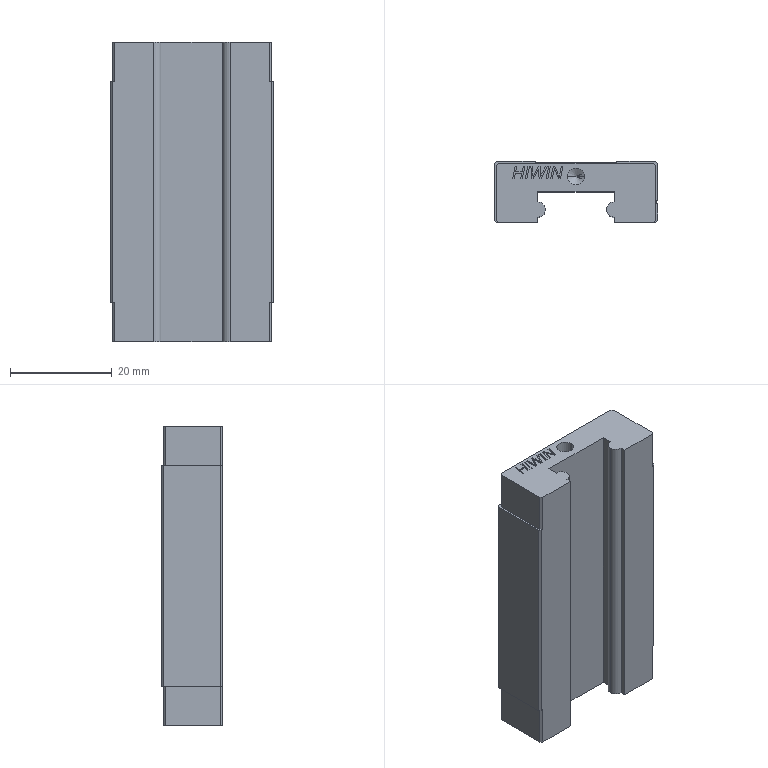Part | STEP file | MGN15H-130-02-cc | 1 solid | 206 faces | box 32 x 12 x 58.8 mm | volume 16948 mm3 | plane 137 | spline 40 | cylinder 17 | cone 12 | commonest cylinder face diameters 3 x11 3.3 x4 0.6 x2